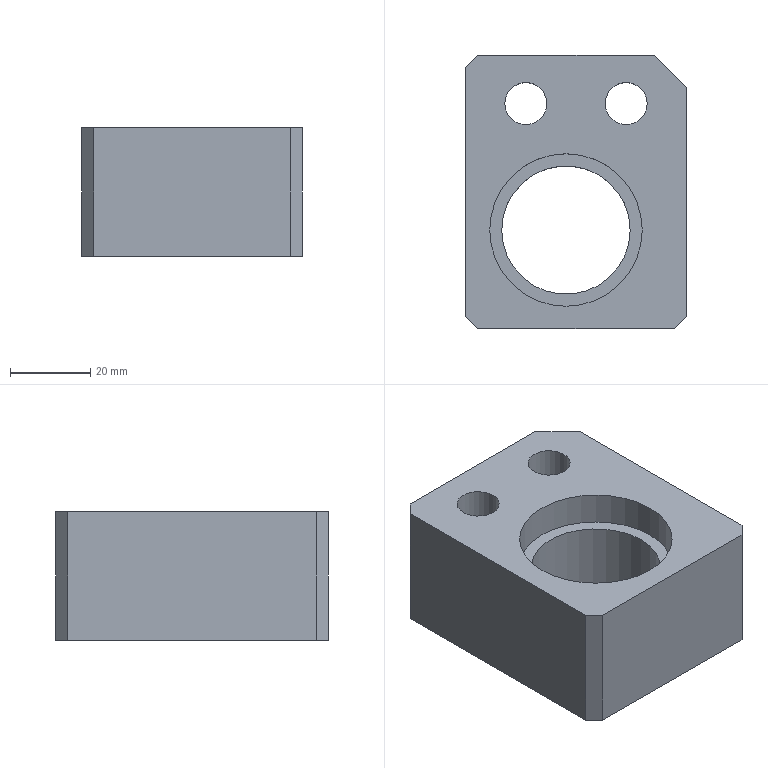Part | STEP file | lll_id3574_x_t | 1 solid | 19 faces | box 55 x 68 x 32 mm | volume 79468 mm3 | plane 13 | cylinder 6 | commonest cylinder face diameters 10.5 x2 17 x2 32 x1 38 x1
STEP:
#1=CARTESIAN_POINT('',(3324.617,-172.788,77.5));
#2=VERTEX_POINT('',#1);
#3=CARTESIAN_POINT('',(3329.867,-172.788,77.5));
#4=DIRECTION('',(0.,0.,1.));
#5=DIRECTION('',(-1.,0.,0.));
#6=AXIS2_PLACEMENT_3D('',#3,#4,#5);
#7=CIRCLE('',#6,5.25);
#8=EDGE_CURVE('',#2,#2,#7,.T.);
#9=ORIENTED_EDGE('',*,*,#8,.T.);
#10=EDGE_LOOP('',(#9));
#11=FACE_BOUND('',#10,.T.);
#12=CARTESIAN_POINT('',(3321.367,-172.788,77.5));
#13=VERTEX_POINT('',#12);
#14=CARTESIAN_POINT('',(3329.867,-172.788,77.5));
#15=DIRECTION('',(0.,0.,1.));
#16=DIRECTION('',(-1.,0.,0.));
#17=AXIS2_PLACEMENT_3D('',#14,#15,#16);
#18=CIRCLE('',#17,8.5);
#19=EDGE_CURVE('',#13,#13,#18,.T.);
#20=ORIENTED_EDGE('',*,*,#19,.F.);
#21=EDGE_LOOP('',(#20));
#22=FACE_BOUND('',#21,.T.);
#23=CARTESIAN_POINT('',(3329.867,-172.788,77.5));
#24=DIRECTION('',(0.,0.,1.));
#25=DIRECTION('',(-1.,0.,0.));
#26=AXIS2_PLACEMENT_3D('',#23,#24,#25);
#27=PLANE('',#26);
#28=ADVANCED_FACE('',(#11,#22),#27,.F.);
#29=CARTESIAN_POINT('',(3320.867,-204.288,84.3));
#30=VERTEX_POINT('',#29);
#31=CARTESIAN_POINT('',(3339.867,-204.288,84.3));
#32=DIRECTION('',(0.,0.,1.));
#33=DIRECTION('',(-1.,0.,0.));
#34=AXIS2_PLACEMENT_3D('',#31,#32,#33);
#35=CIRCLE('',#34,19.);
#36=EDGE_CURVE('',#30,#30,#35,.T.);
#37=ORIENTED_EDGE('',*,*,#36,.T.);
#38=EDGE_LOOP('',(#37));
#39=FACE_BOUND('',#38,.T.);
#40=CARTESIAN_POINT('',(3323.867,-204.288,84.3));
#41=VERTEX_POINT('',#40);
#42=CARTESIAN_POINT('',(3339.867,-204.288,84.3));
#43=DIRECTION('',(0.,0.,1.));
#44=DIRECTION('',(-1.,0.,0.));
#45=AXIS2_PLACEMENT_3D('',#42,#43,#44);
#46=CIRCLE('',#45,16.);
#47=EDGE_CURVE('',#41,#41,#46,.T.);
#48=ORIENTED_EDGE('',*,*,#47,.F.);
#49=EDGE_LOOP('',(#48));
#50=FACE_BOUND('',#49,.T.);
#51=CARTESIAN_POINT('',(3339.867,-195.538,84.3));
#52=DIRECTION('',(0.,0.,-1.));
#53=DIRECTION('',(0.,1.,0.));
#54=AXIS2_PLACEMENT_3D('',#51,#52,#53);
#55=PLANE('',#54);
#56=ADVANCED_FACE('',(#39,#50),#55,.F.);
#57=ORIENTED_EDGE('',*,*,#19,.T.);
#58=EDGE_LOOP('',(#57));
#59=FACE_BOUND('',#58,.T.);
#60=CARTESIAN_POINT('',(3321.367,-172.788,60.5));
#61=VERTEX_POINT('',#60);
#62=CARTESIAN_POINT('',(3329.867,-172.788,60.5));
#63=DIRECTION('',(0.,0.,-1.));
#64=DIRECTION('',(-1.,0.,0.));
#65=AXIS2_PLACEMENT_3D('',#62,#63,#64);
#66=CIRCLE('',#65,8.5);
#67=EDGE_CURVE('',#61,#61,#66,.T.);
#68=ORIENTED_EDGE('',*,*,#67,.T.);
#69=EDGE_LOOP('',(#68));
#70=FACE_BOUND('',#69,.T.);
#71=CARTESIAN_POINT('',(3329.867,-172.788,60.5));
#72=DIRECTION('',(0.,0.,1.));
#73=DIRECTION('',(-1.,0.,0.));
#74=AXIS2_PLACEMENT_3D('',#71,#72,#73);
#75=CYLINDRICAL_SURFACE('',#74,8.5);
#76=ADVANCED_FACE('',(#59,#70),#75,.F.);
#77=CARTESIAN_POINT('',(3369.867,-225.788,60.5));
#78=VERTEX_POINT('',#77);
#79=CARTESIAN_POINT('',(3366.867,-228.788,60.5));
#80=VERTEX_POINT('',#79);
#81=CARTESIAN_POINT('',(3350.685,-244.97,60.5));
#82=DIRECTION('',(-0.7071,-0.7071,0.));
#83=VECTOR('',#82,1.);
#84=LINE('',#81,#83);
#85=EDGE_CURVE('',#78,#80,#84,.T.);
#86=ORIENTED_EDGE('',*,*,#85,.F.);
#87=CARTESIAN_POINT('',(3369.867,-225.788,92.5));
#88=VERTEX_POINT('',#87);
#89=CARTESIAN_POINT('',(3369.867,-225.788,-8.5));
#90=DIRECTION('',(0.,0.,-1.));
#91=VECTOR('',#90,1.);
#92=LINE('',#89,#91);
#93=EDGE_CURVE('',#88,#78,#92,.T.);
#94=ORIENTED_EDGE('',*,*,#93,.F.);
#95=CARTESIAN_POINT('',(3366.867,-228.788,92.5));
#96=VERTEX_POINT('',#95);
#97=CARTESIAN_POINT('',(3350.685,-244.97,92.5));
#98=DIRECTION('',(0.7071,0.7071,0.));
#99=VECTOR('',#98,1.);
#100=LINE('',#97,#99);
#101=EDGE_CURVE('',#96,#88,#100,.T.);
#102=ORIENTED_EDGE('',*,*,#101,.F.);
#103=CARTESIAN_POINT('',(3366.867,-228.788,-8.5));
#104=DIRECTION('',(0.,0.,1.));
#105=VECTOR('',#104,1.);
#106=LINE('',#103,#105);
#107=EDGE_CURVE('',#80,#96,#106,.T.);
#108=ORIENTED_EDGE('',*,*,#107,.F.);
#109=EDGE_LOOP('',(#86,#94,#102,#108));
#110=FACE_OUTER_BOUND('',#109,.T.);
#111=CARTESIAN_POINT('',(3366.867,-228.788,-8.5));
#112=DIRECTION('',(-0.7071,0.7071,0.));
#113=DIRECTION('',(0.,0.,1.));
#114=AXIS2_PLACEMENT_3D('',#111,#112,#113);
#115=PLANE('',#114);
#116=ADVANCED_FACE('',(#110),#115,.F.);
#117=CARTESIAN_POINT('',(3317.867,-228.788,60.5));
#118=VERTEX_POINT('',#117);
#119=CARTESIAN_POINT('',(3276.677,-228.788,60.5));
#120=DIRECTION('',(-1.,0.,0.));
#121=VECTOR('',#120,1.);
#122=LINE('',#119,#121);
#123=EDGE_CURVE('',#80,#118,#122,.T.);
#124=ORIENTED_EDGE('',*,*,#123,.F.);
#125=ORIENTED_EDGE('',*,*,#107,.T.);
#126=CARTESIAN_POINT('',(3317.867,-228.788,92.5));
#127=VERTEX_POINT('',#126);
#128=CARTESIAN_POINT('',(3339.867,-228.788,92.5));
#129=DIRECTION('',(1.,0.,0.));
#130=VECTOR('',#129,1.);
#131=LINE('',#128,#130);
#132=EDGE_CURVE('',#127,#96,#131,.T.);
#133=ORIENTED_EDGE('',*,*,#132,.F.);
#134=CARTESIAN_POINT('',(3317.867,-228.788,-8.5));
#135=DIRECTION('',(0.,0.,1.));
#136=VECTOR('',#135,1.);
#137=LINE('',#134,#136);
#138=EDGE_CURVE('',#118,#127,#137,.T.);
#139=ORIENTED_EDGE('',*,*,#138,.F.);
#140=EDGE_LOOP('',(#124,#125,#133,#139));
#141=FACE_OUTER_BOUND('',#140,.T.);
#142=CARTESIAN_POINT('',(3339.867,-228.788,-8.5));
#143=DIRECTION('',(0.,-1.,0.));
#144=DIRECTION('',(0.,0.,-1.));
#145=AXIS2_PLACEMENT_3D('',#142,#143,#144);
#146=PLANE('',#145);
#147=ADVANCED_FACE('',(#141),#146,.T.);
#148=CARTESIAN_POINT('',(3314.867,-225.788,92.5));
#149=VERTEX_POINT('',#148);
#150=CARTESIAN_POINT('',(3314.867,-225.788,92.5));
#151=DIRECTION('',(-0.7071,0.7071,0.));
#152=VECTOR('',#151,1.);
#153=LINE('',#150,#152);
#154=EDGE_CURVE('',#127,#149,#153,.T.);
#155=ORIENTED_EDGE('',*,*,#154,.T.);
#156=CARTESIAN_POINT('',(3314.867,-225.788,60.5));
#157=VERTEX_POINT('',#156);
#158=CARTESIAN_POINT('',(3314.867,-225.788,-8.5));
#159=DIRECTION('',(0.,0.,-1.));
#160=VECTOR('',#159,1.);
#161=LINE('',#158,#160);
#162=EDGE_CURVE('',#149,#157,#161,.T.);
#163=ORIENTED_EDGE('',*,*,#162,.T.);
#164=CARTESIAN_POINT('',(3319.817,-230.738,60.5));
#165=DIRECTION('',(0.7071,-0.7071,0.));
#166=VECTOR('',#165,1.);
#167=LINE('',#164,#166);
#168=EDGE_CURVE('',#157,#118,#167,.T.);
#169=ORIENTED_EDGE('',*,*,#168,.T.);
#170=ORIENTED_EDGE('',*,*,#138,.T.);
#171=EDGE_LOOP('',(#155,#163,#169,#170));
#172=FACE_OUTER_BOUND('',#171,.T.);
#173=CARTESIAN_POINT('',(3314.867,-225.788,-8.5));
#174=DIRECTION('',(0.7071,0.7071,0.));
#175=DIRECTION('',(-0.7071,0.7071,0.));
#176=AXIS2_PLACEMENT_3D('',#173,#174,#175);
#177=PLANE('',#176);
#178=ADVANCED_FACE('',(#172),#177,.F.);
#179=CARTESIAN_POINT('',(3314.867,-163.788,60.5));
#180=VERTEX_POINT('',#179);
#181=CARTESIAN_POINT('',(3314.867,-178.012,60.5));
#182=DIRECTION('',(0.,1.,0.));
#183=VECTOR('',#182,1.);
#184=LINE('',#181,#183);
#185=EDGE_CURVE('',#157,#180,#184,.T.);
#186=ORIENTED_EDGE('',*,*,#185,.F.);
#187=ORIENTED_EDGE('',*,*,#162,.F.);
#188=CARTESIAN_POINT('',(3314.867,-163.788,92.5));
#189=VERTEX_POINT('',#188);
#190=CARTESIAN_POINT('',(3314.867,-173.063,92.5));
#191=DIRECTION('',(0.,-1.,0.));
#192=VECTOR('',#191,1.);
#193=LINE('',#190,#192);
#194=EDGE_CURVE('',#189,#149,#193,.T.);
#195=ORIENTED_EDGE('',*,*,#194,.F.);
#196=CARTESIAN_POINT('',(3314.867,-163.788,-8.5));
#197=DIRECTION('',(0.,0.,1.));
#198=VECTOR('',#197,1.);
#199=LINE('',#196,#198);
#200=EDGE_CURVE('',#180,#189,#199,.T.);
#201=ORIENTED_EDGE('',*,*,#200,.F.);
#202=EDGE_LOOP('',(#186,#187,#195,#201));
#203=FACE_OUTER_BOUND('',#202,.T.);
#204=CARTESIAN_POINT('',(3314.867,-204.288,-8.5));
#205=DIRECTION('',(-1.,0.,0.));
#206=DIRECTION('',(0.,0.,-1.));
#207=AXIS2_PLACEMENT_3D('',#204,#205,#206);
#208=PLANE('',#207);
#209=ADVANCED_FACE('',(#203),#208,.T.);
#210=CARTESIAN_POINT('',(3317.867,-160.788,92.5));
#211=VERTEX_POINT('',#210);
#212=CARTESIAN_POINT('',(3317.867,-160.788,92.5));
#213=DIRECTION('',(0.7071,0.7071,0.));
#214=VECTOR('',#213,1.);
#215=LINE('',#212,#214);
#216=EDGE_CURVE('',#189,#211,#215,.T.);
#217=ORIENTED_EDGE('',*,*,#216,.T.);
#218=CARTESIAN_POINT('',(3317.867,-160.788,60.5));
#219=VERTEX_POINT('',#218);
#220=CARTESIAN_POINT('',(3317.867,-160.788,-8.5));
#221=DIRECTION('',(0.,0.,-1.));
#222=VECTOR('',#221,1.);
#223=LINE('',#220,#222);
#224=EDGE_CURVE('',#211,#219,#223,.T.);
#225=ORIENTED_EDGE('',*,*,#224,.T.);
#226=CARTESIAN_POINT('',(3317.867,-160.788,60.5));
#227=DIRECTION('',(-0.7071,-0.7071,0.));
#228=VECTOR('',#227,1.);
#229=LINE('',#226,#228);
#230=EDGE_CURVE('',#219,#180,#229,.T.);
#231=ORIENTED_EDGE('',*,*,#230,.T.);
#232=ORIENTED_EDGE('',*,*,#200,.T.);
#233=EDGE_LOOP('',(#217,#225,#231,#232));
#234=FACE_OUTER_BOUND('',#233,.T.);
#235=CARTESIAN_POINT('',(3317.867,-160.788,-8.5));
#236=DIRECTION('',(0.7071,-0.7071,0.));
#237=DIRECTION('',(0.7071,0.7071,0.));
#238=AXIS2_PLACEMENT_3D('',#235,#236,#237);
#239=PLANE('',#238);
#240=ADVANCED_FACE('',(#234),#239,.F.);
#241=CARTESIAN_POINT('',(3361.867,-160.788,92.5));
#242=VERTEX_POINT('',#241);
#243=CARTESIAN_POINT('',(3339.867,-160.788,92.5));
#244=DIRECTION('',(-1.,0.,0.));
#245=VECTOR('',#244,1.);
#246=LINE('',#243,#245);
#247=EDGE_CURVE('',#242,#211,#246,.T.);
#248=ORIENTED_EDGE('',*,*,#247,.F.);
#249=CARTESIAN_POINT('',(3361.867,-160.788,60.5));
#250=VERTEX_POINT('',#249);
#251=CARTESIAN_POINT('',(3361.867,-160.788,-8.5));
#252=DIRECTION('',(0.,0.,-1.));
#253=VECTOR('',#252,1.);
#254=LINE('',#251,#253);
#255=EDGE_CURVE('',#242,#250,#254,.T.);
#256=ORIENTED_EDGE('',*,*,#255,.T.);
#257=CARTESIAN_POINT('',(3276.677,-160.788,60.5));
#258=DIRECTION('',(1.,0.,0.));
#259=VECTOR('',#258,1.);
#260=LINE('',#257,#259);
#261=EDGE_CURVE('',#219,#250,#260,.T.);
#262=ORIENTED_EDGE('',*,*,#261,.F.);
#263=ORIENTED_EDGE('',*,*,#224,.F.);
#264=EDGE_LOOP('',(#248,#256,#262,#263));
#265=FACE_OUTER_BOUND('',#264,.T.);
#266=CARTESIAN_POINT('',(3339.867,-160.788,-8.5));
#267=DIRECTION('',(0.,1.,0.));
#268=DIRECTION('',(0.,0.,1.));
#269=AXIS2_PLACEMENT_3D('',#266,#267,#268);
#270=PLANE('',#269);
#271=ADVANCED_FACE('',(#265),#270,.T.);
#272=CARTESIAN_POINT('',(3369.867,-168.788,92.5));
#273=VERTEX_POINT('',#272);
#274=CARTESIAN_POINT('',(3326.459,-125.38,92.5));
#275=DIRECTION('',(-0.7071,0.7071,0.));
#276=VECTOR('',#275,1.);
#277=LINE('',#274,#276);
#278=EDGE_CURVE('',#273,#242,#277,.T.);
#279=ORIENTED_EDGE('',*,*,#278,.F.);
#280=CARTESIAN_POINT('',(3369.867,-168.788,60.5));
#281=VERTEX_POINT('',#280);
#282=CARTESIAN_POINT('',(3369.867,-168.788,-8.5));
#283=DIRECTION('',(0.,0.,1.));
#284=VECTOR('',#283,1.);
#285=LINE('',#282,#284);
#286=EDGE_CURVE('',#281,#273,#285,.T.);
#287=ORIENTED_EDGE('',*,*,#286,.F.);
#288=CARTESIAN_POINT('',(3331.409,-130.33,60.5));
#289=DIRECTION('',(0.7071,-0.7071,0.));
#290=VECTOR('',#289,1.);
#291=LINE('',#288,#290);
#292=EDGE_CURVE('',#250,#281,#291,.T.);
#293=ORIENTED_EDGE('',*,*,#292,.F.);
#294=ORIENTED_EDGE('',*,*,#255,.F.);
#295=EDGE_LOOP('',(#279,#287,#293,#294));
#296=FACE_OUTER_BOUND('',#295,.T.);
#297=CARTESIAN_POINT('',(3361.867,-160.788,-8.5));
#298=DIRECTION('',(-0.7071,-0.7071,0.));
#299=DIRECTION('',(0.,0.,-1.));
#300=AXIS2_PLACEMENT_3D('',#297,#298,#299);
#301=PLANE('',#300);
#302=ADVANCED_FACE('',(#296),#301,.F.);
#303=CARTESIAN_POINT('',(3369.867,-178.012,60.5));
#304=DIRECTION('',(0.,-1.,0.));
#305=VECTOR('',#304,1.);
#306=LINE('',#303,#305);
#307=EDGE_CURVE('',#281,#78,#306,.T.);
#308=ORIENTED_EDGE('',*,*,#307,.F.);
#309=ORIENTED_EDGE('',*,*,#286,.T.);
#310=CARTESIAN_POINT('',(3369.867,-178.012,92.5));
#311=DIRECTION('',(0.,1.,0.));
#312=VECTOR('',#311,1.);
#313=LINE('',#310,#312);
#314=EDGE_CURVE('',#88,#273,#313,.T.);
#315=ORIENTED_EDGE('',*,*,#314,.F.);
#316=ORIENTED_EDGE('',*,*,#93,.T.);
#317=EDGE_LOOP('',(#308,#309,#315,#316));
#318=FACE_OUTER_BOUND('',#317,.T.);
#319=CARTESIAN_POINT('',(3369.867,-209.238,-8.5));
#320=DIRECTION('',(1.,0.,0.));
#321=DIRECTION('',(0.,0.,1.));
#322=AXIS2_PLACEMENT_3D('',#319,#320,#321);
#323=PLANE('',#322);
#324=ADVANCED_FACE('',(#318),#323,.T.);
#325=CARTESIAN_POINT('',(3324.617,-172.788,92.5));
#326=VERTEX_POINT('',#325);
#327=CARTESIAN_POINT('',(3329.867,-172.788,92.5));
#328=DIRECTION('',(0.,0.,-1.));
#329=DIRECTION('',(-1.,0.,0.));
#330=AXIS2_PLACEMENT_3D('',#327,#328,#329);
#331=CIRCLE('',#330,5.25);
#332=EDGE_CURVE('',#326,#326,#331,.T.);
#333=ORIENTED_EDGE('',*,*,#332,.F.);
#334=EDGE_LOOP('',(#333));
#335=FACE_BOUND('',#334,.T.);
#336=ORIENTED_EDGE('',*,*,#8,.F.);
#337=EDGE_LOOP('',(#336));
#338=FACE_BOUND('',#337,.T.);
#339=CARTESIAN_POINT('',(3329.867,-172.788,160.5));
#340=DIRECTION('',(0.,0.,1.));
#341=DIRECTION('',(-1.,0.,0.));
#342=AXIS2_PLACEMENT_3D('',#339,#340,#341);
#343=CYLINDRICAL_SURFACE('',#342,5.25);
#344=ADVANCED_FACE('',(#335,#338),#343,.F.);
#345=CARTESIAN_POINT('',(3358.867,-204.288,92.5));
#346=VERTEX_POINT('',#345);
#347=CARTESIAN_POINT('',(3339.867,-204.288,92.5));
#348=DIRECTION('',(0.,0.,-1.));
#349=DIRECTION('',(1.,0.,0.));
#350=AXIS2_PLACEMENT_3D('',#347,#348,#349);
#351=CIRCLE('',#350,19.);
#352=EDGE_CURVE('',#346,#346,#351,.T.);
#353=ORIENTED_EDGE('',*,*,#352,.F.);
#354=EDGE_LOOP('',(#353));
#355=FACE_BOUND('',#354,.T.);
#356=ORIENTED_EDGE('',*,*,#36,.F.);
#357=EDGE_LOOP('',(#356));
#358=FACE_BOUND('',#357,.T.);
#359=CARTESIAN_POINT('',(3339.867,-204.288,90.));
#360=DIRECTION('',(0.,0.,-1.));
#361=DIRECTION('',(0.,-1.,0.));
#362=AXIS2_PLACEMENT_3D('',#359,#360,#361);
#363=CYLINDRICAL_SURFACE('',#362,19.);
#364=ADVANCED_FACE('',(#355,#358),#363,.F.);
#365=CARTESIAN_POINT('',(3360.117,-172.788,92.5));
#366=VERTEX_POINT('',#365);
#367=CARTESIAN_POINT('',(3354.867,-172.788,92.5));
#368=DIRECTION('',(0.,0.,1.));
#369=DIRECTION('',(1.,0.,0.));
#370=AXIS2_PLACEMENT_3D('',#367,#368,#369);
#371=CIRCLE('',#370,5.25);
#372=EDGE_CURVE('',#366,#366,#371,.T.);
#373=ORIENTED_EDGE('',*,*,#372,.F.);
#374=EDGE_LOOP('',(#373));
#375=FACE_BOUND('',#374,.T.);
#376=ORIENTED_EDGE('',*,*,#352,.T.);
#377=EDGE_LOOP('',(#376));
#378=FACE_BOUND('',#377,.T.);
#379=ORIENTED_EDGE('',*,*,#332,.T.);
#380=EDGE_LOOP('',(#379));
#381=FACE_BOUND('',#380,.T.);
#382=ORIENTED_EDGE('',*,*,#314,.T.);
#383=ORIENTED_EDGE('',*,*,#278,.T.);
#384=ORIENTED_EDGE('',*,*,#247,.T.);
#385=ORIENTED_EDGE('',*,*,#216,.F.);
#386=ORIENTED_EDGE('',*,*,#194,.T.);
#387=ORIENTED_EDGE('',*,*,#154,.F.);
#388=ORIENTED_EDGE('',*,*,#132,.T.);
#389=ORIENTED_EDGE('',*,*,#101,.T.);
#390=EDGE_LOOP('',(#382,#383,#384,#385,#386,#387,#388,#389));
#391=FACE_BOUND('',#390,.T.);
#392=CARTESIAN_POINT('',(3271.727,-173.063,92.5));
#393=DIRECTION('',(0.,0.,1.));
#394=DIRECTION('',(-1.,0.,0.));
#395=AXIS2_PLACEMENT_3D('',#392,#393,#394);
#396=PLANE('',#395);
#397=ADVANCED_FACE('',(#375,#378,#381,#391),#396,.T.);
#398=CARTESIAN_POINT('',(3355.867,-204.288,60.5));
#399=VERTEX_POINT('',#398);
#400=CARTESIAN_POINT('',(3339.867,-204.288,60.5));
#401=DIRECTION('',(0.,0.,1.));
#402=DIRECTION('',(1.,0.,0.));
#403=AXIS2_PLACEMENT_3D('',#400,#401,#402);
#404=CIRCLE('',#403,16.);
#405=EDGE_CURVE('',#399,#399,#404,.T.);
#406=ORIENTED_EDGE('',*,*,#405,.F.);
#407=EDGE_LOOP('',(#406));
#408=FACE_BOUND('',#407,.T.);
#409=ORIENTED_EDGE('',*,*,#47,.T.);
#410=EDGE_LOOP('',(#409));
#411=FACE_BOUND('',#410,.T.);
#412=CARTESIAN_POINT('',(3339.867,-204.288,44.8));
#413=DIRECTION('',(0.,0.,-1.));
#414=DIRECTION('',(0.,-1.,0.));
#415=AXIS2_PLACEMENT_3D('',#412,#413,#414);
#416=CYLINDRICAL_SURFACE('',#415,16.);
#417=ADVANCED_FACE('',(#408,#411),#416,.F.);
#418=CARTESIAN_POINT('',(3363.367,-172.788,60.5));
#419=VERTEX_POINT('',#418);
#420=CARTESIAN_POINT('',(3354.867,-172.788,60.5));
#421=DIRECTION('',(0.,0.,-1.));
#422=DIRECTION('',(1.,0.,0.));
#423=AXIS2_PLACEMENT_3D('',#420,#421,#422);
#424=CIRCLE('',#423,8.5);
#425=EDGE_CURVE('',#419,#419,#424,.T.);
#426=ORIENTED_EDGE('',*,*,#425,.F.);
#427=EDGE_LOOP('',(#426));
#428=FACE_BOUND('',#427,.T.);
#429=ORIENTED_EDGE('',*,*,#405,.T.);
#430=EDGE_LOOP('',(#429));
#431=FACE_BOUND('',#430,.T.);
#432=ORIENTED_EDGE('',*,*,#261,.T.);
#433=ORIENTED_EDGE('',*,*,#292,.T.);
#434=ORIENTED_EDGE('',*,*,#307,.T.);
#435=ORIENTED_EDGE('',*,*,#85,.T.);
#436=ORIENTED_EDGE('',*,*,#123,.T.);
#437=ORIENTED_EDGE('',*,*,#168,.F.);
#438=ORIENTED_EDGE('',*,*,#185,.T.);
#439=ORIENTED_EDGE('',*,*,#230,.F.);
#440=EDGE_LOOP('',(#432,#433,#434,#435,#436,#437,#438,#439));
#441=FACE_BOUND('',#440,.T.);
#442=ORIENTED_EDGE('',*,*,#67,.F.);
#443=EDGE_LOOP('',(#442));
#444=FACE_BOUND('',#443,.T.);
#445=CARTESIAN_POINT('',(3276.677,-178.012,60.5));
#446=DIRECTION('',(0.,0.,1.));
#447=DIRECTION('',(-1.,0.,0.));
#448=AXIS2_PLACEMENT_3D('',#445,#446,#447);
#449=PLANE('',#448);
#450=ADVANCED_FACE('',(#428,#431,#441,#444),#449,.F.);
#451=CARTESIAN_POINT('',(3360.117,-172.788,77.5));
#452=VERTEX_POINT('',#451);
#453=CARTESIAN_POINT('',(3354.867,-172.788,77.5));
#454=DIRECTION('',(0.,0.,1.));
#455=DIRECTION('',(1.,0.,0.));
#456=AXIS2_PLACEMENT_3D('',#453,#454,#455);
#457=CIRCLE('',#456,5.25);
#458=EDGE_CURVE('',#452,#452,#457,.T.);
#459=ORIENTED_EDGE('',*,*,#458,.T.);
#460=EDGE_LOOP('',(#459));
#461=FACE_BOUND('',#460,.T.);
#462=CARTESIAN_POINT('',(3363.367,-172.788,77.5));
#463=VERTEX_POINT('',#462);
#464=CARTESIAN_POINT('',(3354.867,-172.788,77.5));
#465=DIRECTION('',(0.,0.,1.));
#466=DIRECTION('',(1.,0.,0.));
#467=AXIS2_PLACEMENT_3D('',#464,#465,#466);
#468=CIRCLE('',#467,8.5);
#469=EDGE_CURVE('',#463,#463,#468,.T.);
#470=ORIENTED_EDGE('',*,*,#469,.F.);
#471=EDGE_LOOP('',(#470));
#472=FACE_BOUND('',#471,.T.);
#473=CARTESIAN_POINT('',(3354.867,-172.788,77.5));
#474=DIRECTION('',(0.,0.,1.));
#475=DIRECTION('',(1.,0.,0.));
#476=AXIS2_PLACEMENT_3D('',#473,#474,#475);
#477=PLANE('',#476);
#478=ADVANCED_FACE('',(#461,#472),#477,.F.);
#479=ORIENTED_EDGE('',*,*,#372,.T.);
#480=EDGE_LOOP('',(#479));
#481=FACE_BOUND('',#480,.T.);
#482=ORIENTED_EDGE('',*,*,#458,.F.);
#483=EDGE_LOOP('',(#482));
#484=FACE_BOUND('',#483,.T.);
#485=CARTESIAN_POINT('',(3354.867,-172.788,160.5));
#486=DIRECTION('',(0.,0.,1.));
#487=DIRECTION('',(1.,0.,0.));
#488=AXIS2_PLACEMENT_3D('',#485,#486,#487);
#489=CYLINDRICAL_SURFACE('',#488,5.25);
#490=ADVANCED_FACE('',(#481,#484),#489,.F.);
#491=ORIENTED_EDGE('',*,*,#469,.T.);
#492=EDGE_LOOP('',(#491));
#493=FACE_BOUND('',#492,.T.);
#494=ORIENTED_EDGE('',*,*,#425,.T.);
#495=EDGE_LOOP('',(#494));
#496=FACE_BOUND('',#495,.T.);
#497=CARTESIAN_POINT('',(3354.867,-172.788,60.5));
#498=DIRECTION('',(0.,0.,1.));
#499=DIRECTION('',(1.,0.,0.));
#500=AXIS2_PLACEMENT_3D('',#497,#498,#499);
#501=CYLINDRICAL_SURFACE('',#500,8.5);
#502=ADVANCED_FACE('',(#493,#496),#501,.F.);
#503=CLOSED_SHELL('',(#28,#56,#76,#116,#147,#178,#209,#240,#271,#302,#324,#344,#364,#397,#417,#450,#478,#490,#502));
#504=MANIFOLD_SOLID_BREP('',#503);
#505=(LENGTH_UNIT()NAMED_UNIT(*)SI_UNIT(.MILLI.,.METRE.));
#506=UNCERTAINTY_MEASURE_WITH_UNIT(LENGTH_MEASURE(0.00002),#505,'','');
#507=(NAMED_UNIT(*)PLANE_ANGLE_UNIT()SI_UNIT($,.RADIAN.));
#508=PLANE_ANGLE_MEASURE_WITH_UNIT(PLANE_ANGLE_MEASURE(0.01745),#507);
#509=DIMENSIONAL_EXPONENTS(0.,0.,0.,0.,0.,0.,0.);
#510=(CONVERSION_BASED_UNIT('DEGREE',#508)NAMED_UNIT(#509)PLANE_ANGLE_UNIT());
#511=(NAMED_UNIT(*)SI_UNIT($,.STERADIAN.)SOLID_ANGLE_UNIT());
#512=(GEOMETRIC_REPRESENTATION_CONTEXT(3)GLOBAL_UNCERTAINTY_ASSIGNED_CONTEXT((#506))GLOBAL_UNIT_ASSIGNED_CONTEXT((#505,#510,#511))REPRESENTATION_CONTEXT('',''));
#513=ADVANCED_BREP_SHAPE_REPRESENTATION('',(#504),#512);